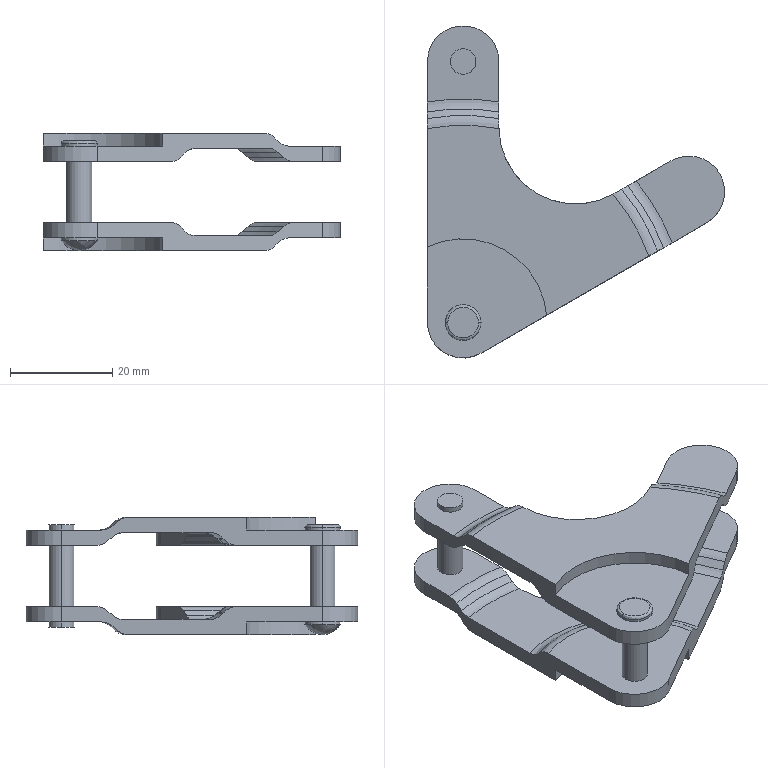Part | STEP file | Sceond_200_APVM0 -4 | 1 solid | 85 faces | box 58.167 x 65 x 23 mm | volume 11402 mm3 | plane 27 | cylinder 24 | spline 23 | cone 11 | commonest cylinder face diameters 5 x8 14 x8 7 x4 30 x2 32.8 x2